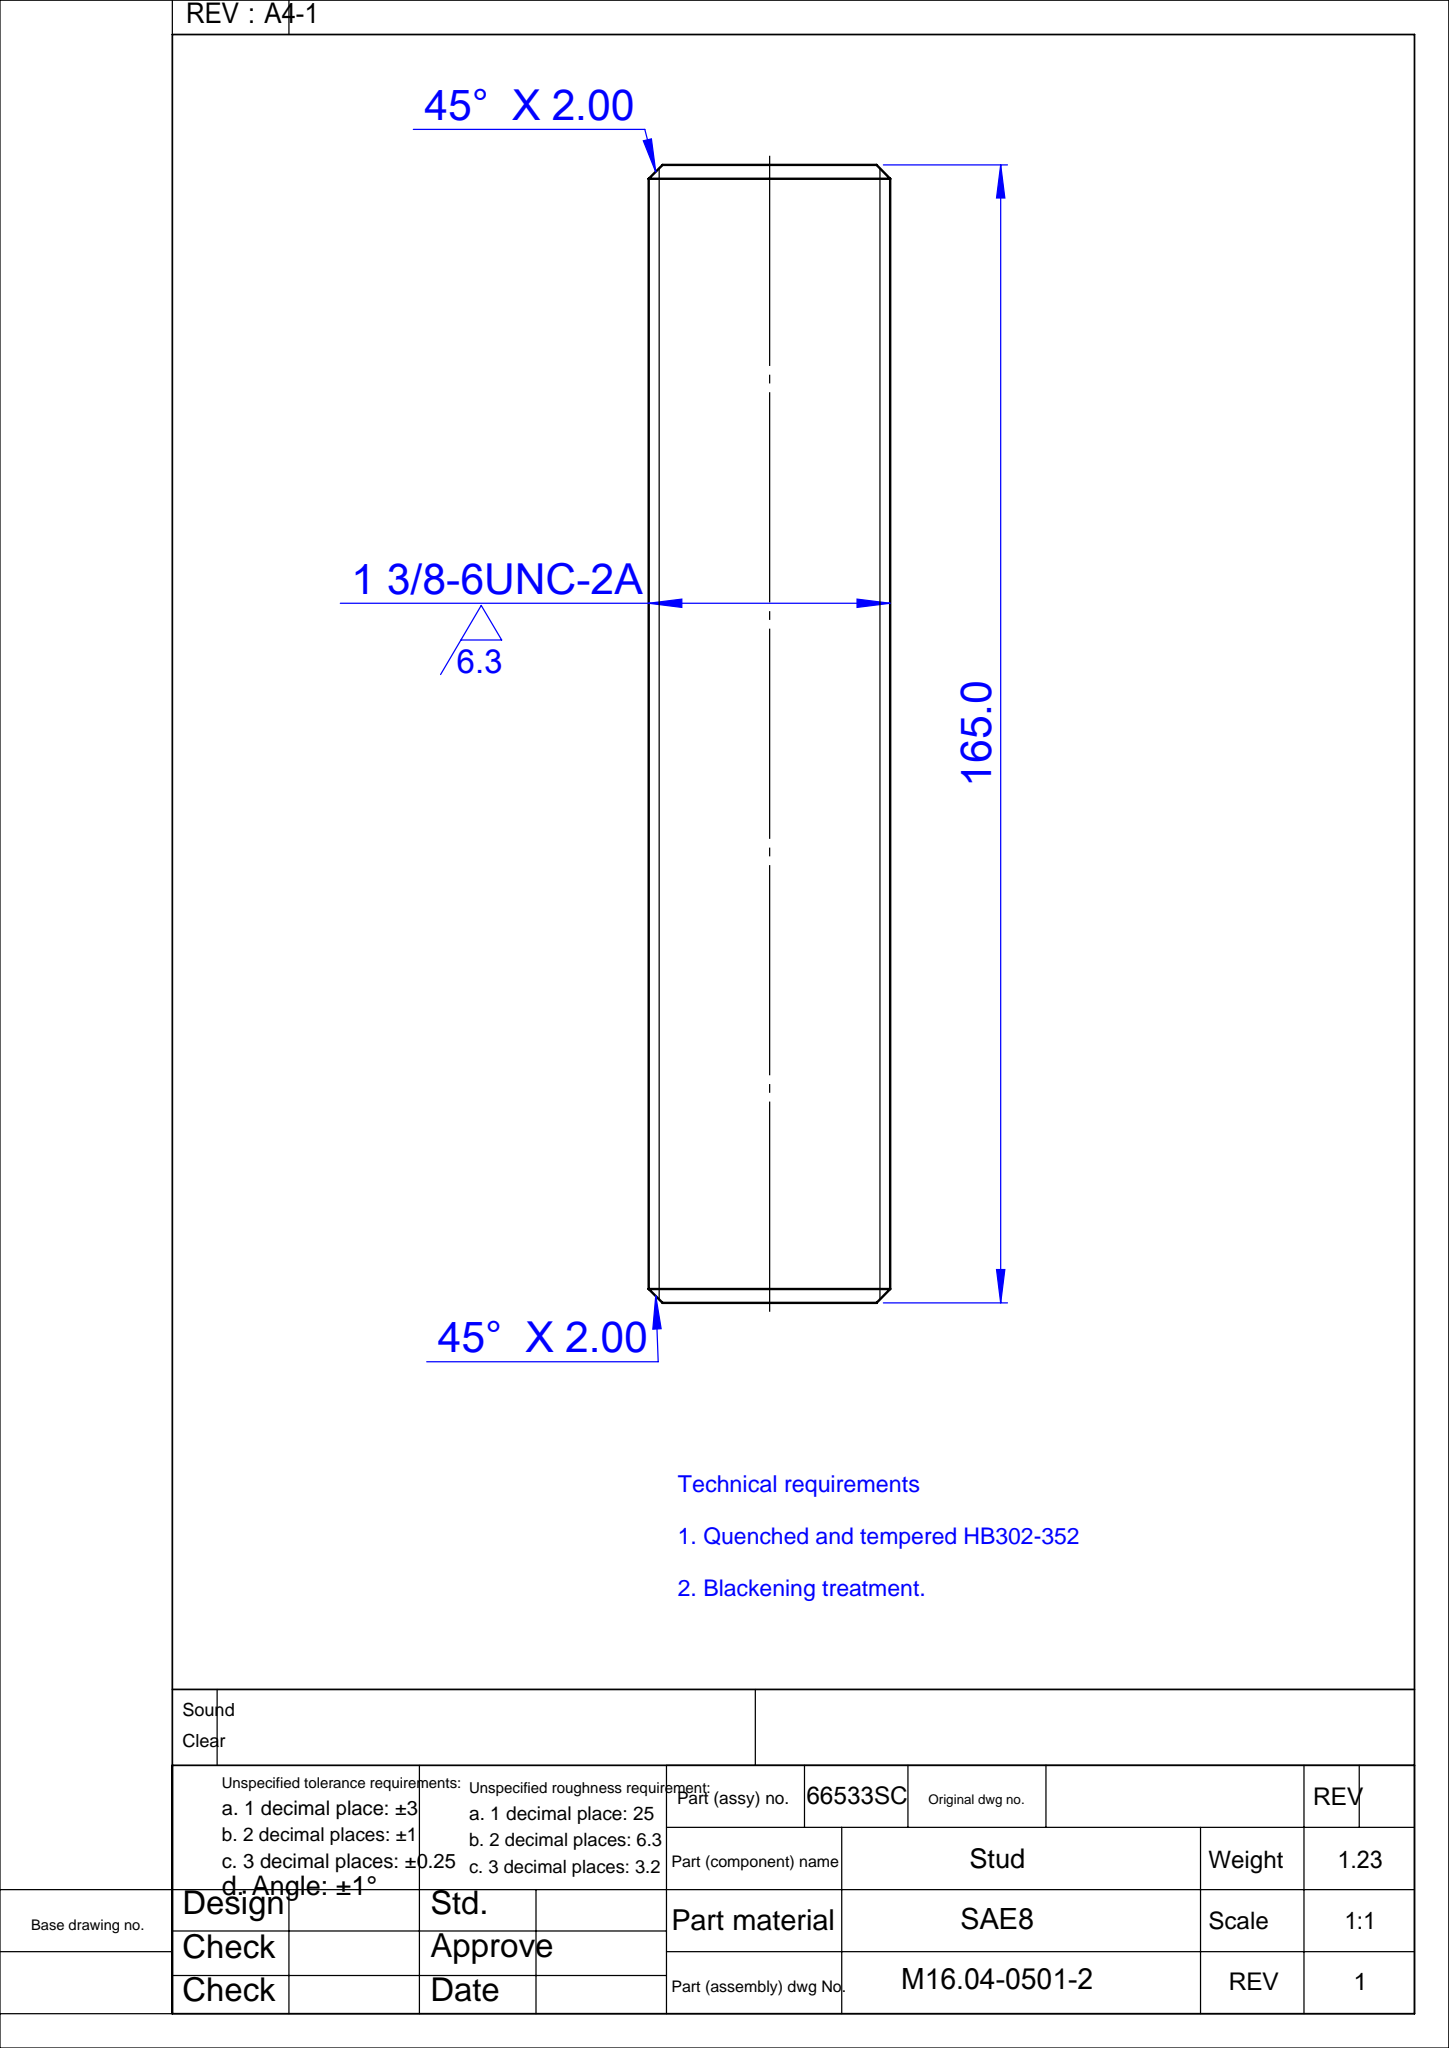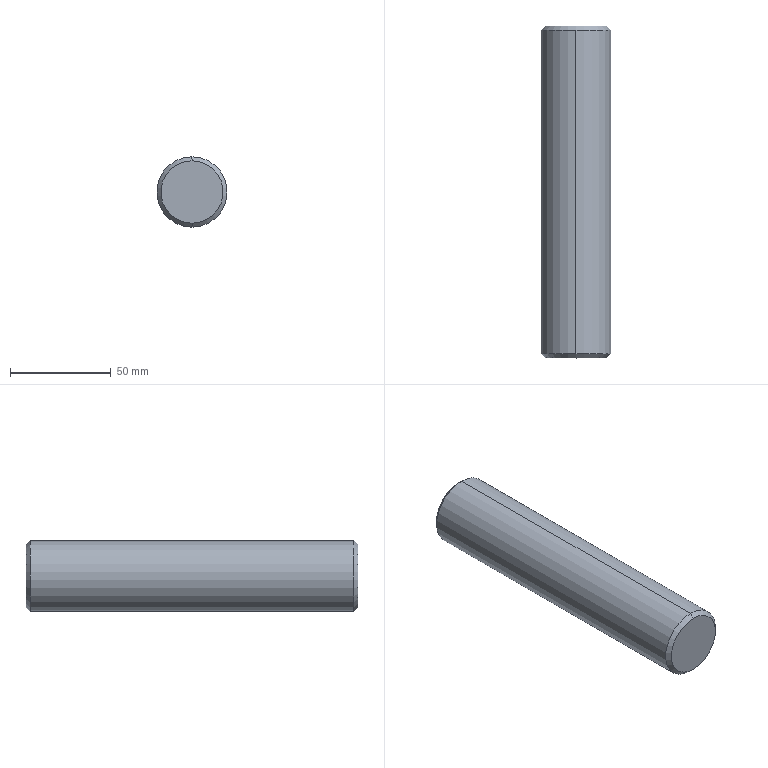Part | SolidWorks | features Chamfer 1, Revolution 1 | 1 solid | 8 faces | box 35 x 165 x 35 mm | volume 158326 mm3 | cone 4 | cylinder 2 | plane 2 | commonest cylinder face diameters 35 x2
STEP:
#1=CARTESIAN_POINT('',(0.,165.,15.5));
#2=VERTEX_POINT('',#1);
#3=CARTESIAN_POINT('',(0.,165.,-15.5));
#4=VERTEX_POINT('',#3);
#5=CARTESIAN_POINT('',(0.,165.,0.));
#6=DIRECTION('',(0.,1.,0.));
#7=DIRECTION('',(0.,0.,1.));
#8=AXIS2_PLACEMENT_3D('',#5,#6,#7);
#9=CIRCLE('',#8,15.5);
#10=EDGE_CURVE('',#2,#4,#9,.T.);
#11=ORIENTED_EDGE('',*,*,#10,.F.);
#12=CARTESIAN_POINT('',(0.,163.,17.5));
#13=VERTEX_POINT('',#12);
#14=CARTESIAN_POINT('',(0.,165.,15.5));
#15=DIRECTION('',(0.,-0.7071,0.7071));
#16=VECTOR('',#15,1000.);
#17=LINE('',#14,#16);
#18=EDGE_CURVE('',#2,#13,#17,.T.);
#19=ORIENTED_EDGE('',*,*,#18,.T.);
#20=CARTESIAN_POINT('',(0.,163.,-17.5));
#21=VERTEX_POINT('',#20);
#22=CARTESIAN_POINT('',(0.,163.,0.));
#23=DIRECTION('',(0.,-1.,0.));
#24=DIRECTION('',(0.,0.,1.));
#25=AXIS2_PLACEMENT_3D('',#22,#23,#24);
#26=CIRCLE('',#25,17.5);
#27=EDGE_CURVE('',#21,#13,#26,.T.);
#28=ORIENTED_EDGE('',*,*,#27,.F.);
#29=CARTESIAN_POINT('',(0.,165.,-15.5));
#30=DIRECTION('',(0.,-0.7071,-0.7071));
#31=VECTOR('',#30,1000.);
#32=LINE('',#29,#31);
#33=EDGE_CURVE('',#4,#21,#32,.T.);
#34=ORIENTED_EDGE('',*,*,#33,.F.);
#35=EDGE_LOOP('',(#11,#19,#28,#34));
#36=FACE_OUTER_BOUND('',#35,.T.);
#37=CARTESIAN_POINT('',(0.,165.,0.));
#38=DIRECTION('',(0.,-1.,0.));
#39=DIRECTION('',(0.,0.,-1.));
#40=AXIS2_PLACEMENT_3D('',#37,#38,#39);
#41=CONICAL_SURFACE('',#40,15.5,0.7854);
#42=ADVANCED_FACE('',(#36),#41,.T.);
#43=CARTESIAN_POINT('',(0.,0.,-15.5));
#44=VERTEX_POINT('',#43);
#45=CARTESIAN_POINT('',(0.,0.,15.5));
#46=VERTEX_POINT('',#45);
#47=CARTESIAN_POINT('',(0.,0.,0.));
#48=DIRECTION('',(0.,-1.,0.));
#49=DIRECTION('',(0.,0.,-1.));
#50=AXIS2_PLACEMENT_3D('',#47,#48,#49);
#51=CIRCLE('',#50,15.5);
#52=EDGE_CURVE('',#44,#46,#51,.T.);
#53=ORIENTED_EDGE('',*,*,#52,.F.);
#54=CARTESIAN_POINT('',(0.,2.,-17.5));
#55=VERTEX_POINT('',#54);
#56=CARTESIAN_POINT('',(0.,2.,-17.5));
#57=DIRECTION('',(0.,0.7071,-0.7071));
#58=VECTOR('',#57,1000.);
#59=LINE('',#56,#58);
#60=EDGE_CURVE('',#44,#55,#59,.T.);
#61=ORIENTED_EDGE('',*,*,#60,.T.);
#62=CARTESIAN_POINT('',(0.,2.,17.5));
#63=VERTEX_POINT('',#62);
#64=CARTESIAN_POINT('',(0.,2.,0.));
#65=DIRECTION('',(0.,1.,0.));
#66=DIRECTION('',(0.,0.,-1.));
#67=AXIS2_PLACEMENT_3D('',#64,#65,#66);
#68=CIRCLE('',#67,17.5);
#69=EDGE_CURVE('',#63,#55,#68,.T.);
#70=ORIENTED_EDGE('',*,*,#69,.F.);
#71=CARTESIAN_POINT('',(0.,2.,17.5));
#72=DIRECTION('',(0.,0.7071,0.7071));
#73=VECTOR('',#72,1000.);
#74=LINE('',#71,#73);
#75=EDGE_CURVE('',#46,#63,#74,.T.);
#76=ORIENTED_EDGE('',*,*,#75,.F.);
#77=EDGE_LOOP('',(#53,#61,#70,#76));
#78=FACE_OUTER_BOUND('',#77,.T.);
#79=CARTESIAN_POINT('',(0.,2.,0.));
#80=DIRECTION('',(0.,1.,0.));
#81=DIRECTION('',(0.,0.,1.));
#82=AXIS2_PLACEMENT_3D('',#79,#80,#81);
#83=CONICAL_SURFACE('',#82,17.5,0.7854);
#84=ADVANCED_FACE('',(#78),#83,.T.);
#85=ORIENTED_EDGE('',*,*,#69,.T.);
#86=CARTESIAN_POINT('',(0.,158.861,-17.5));
#87=DIRECTION('',(0.,1.,0.));
#88=VECTOR('',#87,1000.);
#89=LINE('',#86,#88);
#90=EDGE_CURVE('',#55,#21,#89,.T.);
#91=ORIENTED_EDGE('',*,*,#90,.T.);
#92=ORIENTED_EDGE('',*,*,#27,.T.);
#93=CARTESIAN_POINT('',(0.,158.861,17.5));
#94=DIRECTION('',(0.,1.,0.));
#95=VECTOR('',#94,1000.);
#96=LINE('',#93,#95);
#97=EDGE_CURVE('',#63,#13,#96,.T.);
#98=ORIENTED_EDGE('',*,*,#97,.F.);
#99=EDGE_LOOP('',(#85,#91,#92,#98));
#100=FACE_OUTER_BOUND('',#99,.T.);
#101=CARTESIAN_POINT('',(0.,158.861,0.));
#102=DIRECTION('',(0.,1.,0.));
#103=DIRECTION('',(0.,0.,1.));
#104=AXIS2_PLACEMENT_3D('',#101,#102,#103);
#105=CYLINDRICAL_SURFACE('',#104,17.5);
#106=ADVANCED_FACE('',(#100),#105,.T.);
#107=CARTESIAN_POINT('',(0.,165.,0.));
#108=DIRECTION('',(0.,1.,0.));
#109=DIRECTION('',(0.,0.,1.));
#110=AXIS2_PLACEMENT_3D('',#107,#108,#109);
#111=CIRCLE('',#110,15.5);
#112=EDGE_CURVE('',#4,#2,#111,.T.);
#113=ORIENTED_EDGE('',*,*,#112,.T.);
#114=ORIENTED_EDGE('',*,*,#10,.T.);
#115=EDGE_LOOP('',(#113,#114));
#116=FACE_OUTER_BOUND('',#115,.T.);
#117=CARTESIAN_POINT('',(0.,165.,0.));
#118=DIRECTION('',(0.,1.,0.));
#119=DIRECTION('',(0.,0.,1.));
#120=AXIS2_PLACEMENT_3D('',#117,#118,#119);
#121=PLANE('',#120);
#122=ADVANCED_FACE('',(#116),#121,.T.);
#123=ORIENTED_EDGE('',*,*,#90,.F.);
#124=CARTESIAN_POINT('',(0.,2.,0.));
#125=DIRECTION('',(0.,1.,0.));
#126=DIRECTION('',(0.,0.,-1.));
#127=AXIS2_PLACEMENT_3D('',#124,#125,#126);
#128=CIRCLE('',#127,17.5);
#129=EDGE_CURVE('',#55,#63,#128,.T.);
#130=ORIENTED_EDGE('',*,*,#129,.T.);
#131=ORIENTED_EDGE('',*,*,#97,.T.);
#132=CARTESIAN_POINT('',(0.,163.,0.));
#133=DIRECTION('',(0.,-1.,0.));
#134=DIRECTION('',(0.,0.,1.));
#135=AXIS2_PLACEMENT_3D('',#132,#133,#134);
#136=CIRCLE('',#135,17.5);
#137=EDGE_CURVE('',#13,#21,#136,.T.);
#138=ORIENTED_EDGE('',*,*,#137,.T.);
#139=EDGE_LOOP('',(#123,#130,#131,#138));
#140=FACE_OUTER_BOUND('',#139,.T.);
#141=CARTESIAN_POINT('',(0.,158.861,0.));
#142=DIRECTION('',(0.,1.,0.));
#143=DIRECTION('',(0.,0.,1.));
#144=AXIS2_PLACEMENT_3D('',#141,#142,#143);
#145=CYLINDRICAL_SURFACE('',#144,17.5);
#146=ADVANCED_FACE('',(#140),#145,.T.);
#147=CARTESIAN_POINT('',(0.,0.,0.));
#148=DIRECTION('',(0.,-1.,0.));
#149=DIRECTION('',(0.,0.,-1.));
#150=AXIS2_PLACEMENT_3D('',#147,#148,#149);
#151=CIRCLE('',#150,15.5);
#152=EDGE_CURVE('',#46,#44,#151,.T.);
#153=ORIENTED_EDGE('',*,*,#152,.T.);
#154=ORIENTED_EDGE('',*,*,#52,.T.);
#155=EDGE_LOOP('',(#153,#154));
#156=FACE_OUTER_BOUND('',#155,.T.);
#157=CARTESIAN_POINT('',(0.,0.,0.));
#158=DIRECTION('',(0.,-1.,0.));
#159=DIRECTION('',(0.,0.,-1.));
#160=AXIS2_PLACEMENT_3D('',#157,#158,#159);
#161=PLANE('',#160);
#162=ADVANCED_FACE('',(#156),#161,.T.);
#163=ORIENTED_EDGE('',*,*,#60,.F.);
#164=ORIENTED_EDGE('',*,*,#152,.F.);
#165=ORIENTED_EDGE('',*,*,#75,.T.);
#166=ORIENTED_EDGE('',*,*,#129,.F.);
#167=EDGE_LOOP('',(#163,#164,#165,#166));
#168=FACE_OUTER_BOUND('',#167,.T.);
#169=CARTESIAN_POINT('',(0.,2.,0.));
#170=DIRECTION('',(0.,1.,0.));
#171=DIRECTION('',(0.,0.,1.));
#172=AXIS2_PLACEMENT_3D('',#169,#170,#171);
#173=CONICAL_SURFACE('',#172,17.5,0.7854);
#174=ADVANCED_FACE('',(#168),#173,.T.);
#175=ORIENTED_EDGE('',*,*,#18,.F.);
#176=ORIENTED_EDGE('',*,*,#112,.F.);
#177=ORIENTED_EDGE('',*,*,#33,.T.);
#178=ORIENTED_EDGE('',*,*,#137,.F.);
#179=EDGE_LOOP('',(#175,#176,#177,#178));
#180=FACE_OUTER_BOUND('',#179,.T.);
#181=CARTESIAN_POINT('',(0.,165.,0.));
#182=DIRECTION('',(0.,-1.,0.));
#183=DIRECTION('',(0.,0.,-1.));
#184=AXIS2_PLACEMENT_3D('',#181,#182,#183);
#185=CONICAL_SURFACE('',#184,15.5,0.7854);
#186=ADVANCED_FACE('',(#180),#185,.T.);
#187=CLOSED_SHELL('',(#42,#84,#106,#122,#146,#162,#174,#186));
#188=MANIFOLD_SOLID_BREP('',#187);
#189=CARTESIAN_POINT('',(0.,0.,0.));
#190=DIRECTION('',(0.,0.,1.));
#191=DIRECTION('',(1.,0.,0.));
#192=AXIS2_PLACEMENT_3D('',#189,#190,#191);
#193=(LENGTH_UNIT()NAMED_UNIT(*)SI_UNIT(.MILLI.,.METRE.));
#194=UNCERTAINTY_MEASURE_WITH_UNIT(LENGTH_MEASURE(0.00001),#193,'','');
#195=(NAMED_UNIT(*)PLANE_ANGLE_UNIT()SI_UNIT($,.RADIAN.));
#196=(NAMED_UNIT(*)SI_UNIT($,.STERADIAN.)SOLID_ANGLE_UNIT());
#197=(GEOMETRIC_REPRESENTATION_CONTEXT(3)GLOBAL_UNCERTAINTY_ASSIGNED_CONTEXT((#194))GLOBAL_UNIT_ASSIGNED_CONTEXT((#193,#195,#196))REPRESENTATION_CONTEXT('',''));
#198=ADVANCED_BREP_SHAPE_REPRESENTATION('',(#188,#192),#197);